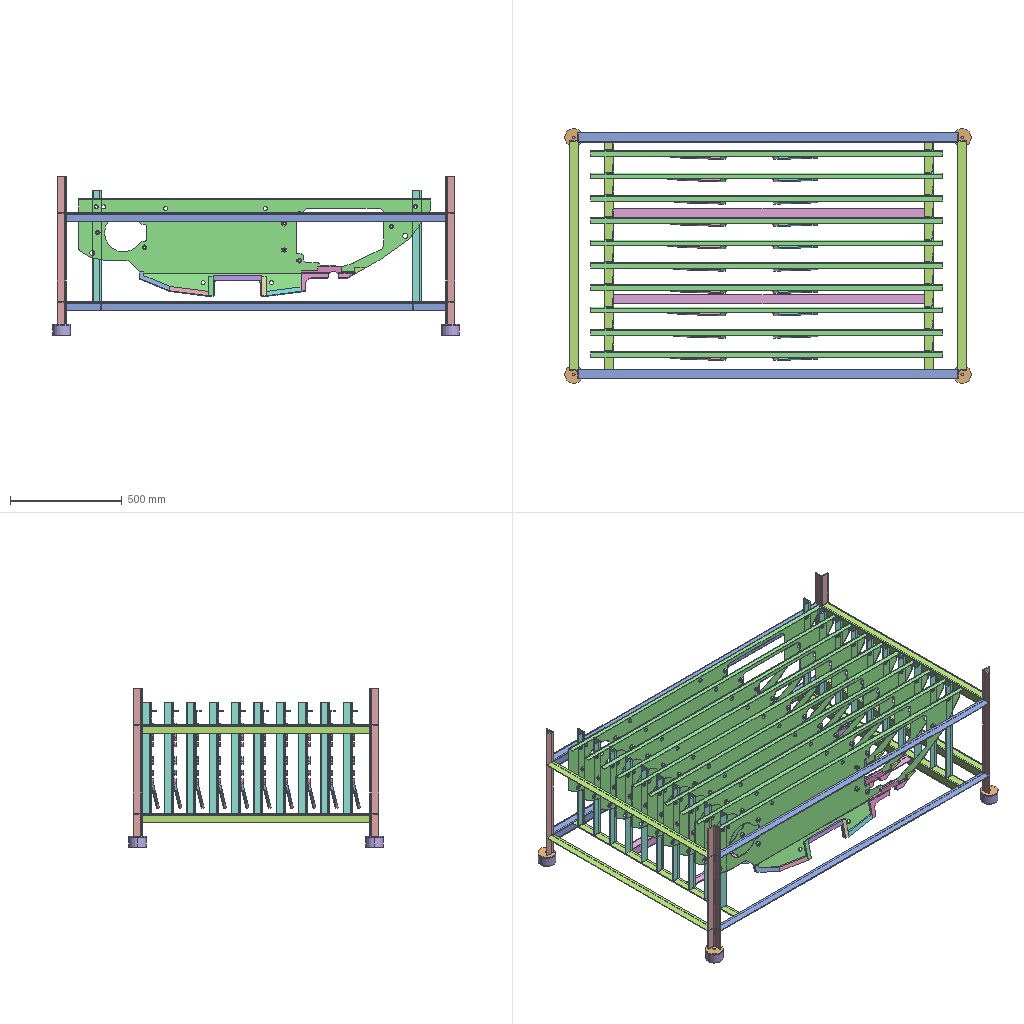Assembly | SolidWorks | 9 different items | 55 placed | box 1820 x 1139 x 710 mm
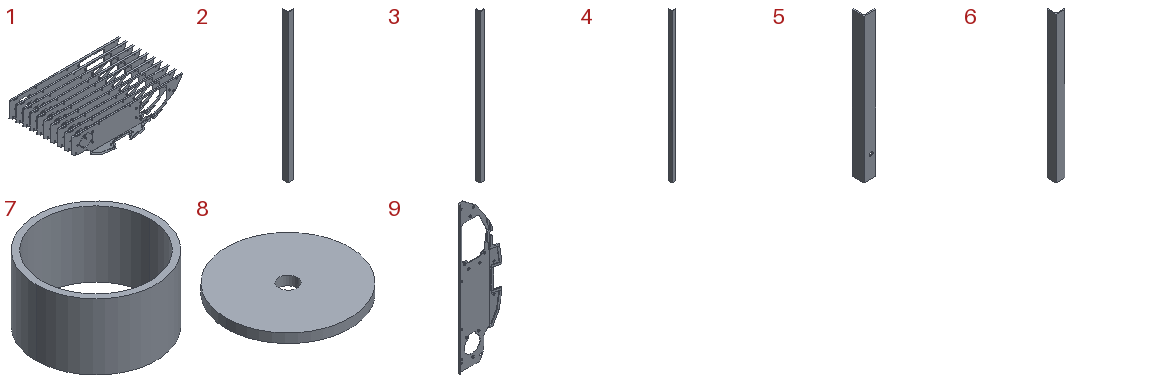Parts list (item | name | quantity | parent item | size | volume | features):
1 | (subassembly) | x1 | - | - | - | features ReferencePattern 9, LocalLPattern 1
2 | - | x6 | - | 40 x 40 x 1020 mm | 314774 mm3 | features Extrusion 1
3 | - | x2 | - | 40 x 40 x 1389 mm | 428648 mm3 | features Extrusion 1
4 | - | x4 | - | 40 x 40 x 1700 mm | 524623 mm3 | features Extrusion 1
5 | - | x20 | - | 40 x 40 x 500 mm | 153770 mm3 | features Extrusion 1, ICE 1
6 | - | x4 | - | 40 x 40 x 660 mm | 203677 mm3 | features Extrusion 1
7 | - | x4 | - | 80 x 80 x 44 mm | 42022 mm3 | features Extrusion 1
8 | - | x4 | - | 80 x 80 x 6 mm | 29481 mm3 | features FlatPattern 1, SMBaseFlange 1, SheetMetal 1
9 | - | x10 | in 1 | - | - | features BaseBody 17, RefSurface 8
Mates (type | each side: item.copy, entity, surface, feature):
Coincident | 6.1 face plane Boss-Extrude1 | 4.1 face plane Boss-Extrude1 | 2 times
DistanceDim | 6.1 face plane Boss-Extrude1 | 4.1 face plane Boss-Extrude1
Coincident | 6.1 face plane Boss-Extrude1 | 2.1 face plane Boss-Extrude1 | 2 times
Coincident | 4.1 face plane Boss-Extrude1 | 2.1 face plane Boss-Extrude1
Coincident | 2.1 face plane Boss-Extrude1 | 6.2 face plane Boss-Extrude1 | 2 times
Coincident | 6.1 face plane Boss-Extrude1 | 6.2 face plane Boss-Extrude1
Coincident | 6.2 face plane Boss-Extrude1 | 4.2 face plane Boss-Extrude1 | 2 times
Coincident | 2.1 face plane Boss-Extrude1 | 4.2 face plane Boss-Extrude1
Coincident | 4.2 face plane Boss-Extrude1 | 6.3 face plane Boss-Extrude1 | 2 times
Coincident | 6.2 face plane Boss-Extrude1 | 6.3 face plane Boss-Extrude1
Coincident | 6.3 face plane Boss-Extrude1 | 2.2 face plane Boss-Extrude1 | 2 times
Coincident | 4.2 face plane Boss-Extrude1 | 2.2 face plane Boss-Extrude1
Coincident | 2.2 face plane Boss-Extrude1 | 6.4 face plane Boss-Extrude1
Coincident | 4.1 face plane Boss-Extrude1 | 6.4 face plane Boss-Extrude1
Coincident | 6.3 face plane Boss-Extrude1 | 6.4 face plane Boss-Extrude1
Coincident | 4.1 face plane Boss-Extrude1 | 2.3 face plane Boss-Extrude1 | 2 times
DistanceDim | 2.1 face plane Boss-Extrude1 | 2.3 face plane Boss-Extrude1
Coincident | 2.2 face plane Boss-Extrude1 | 2.4 face plane Boss-Extrude1
DistanceDim | 2.2 face plane Boss-Extrude1 | 2.4 face plane Boss-Extrude1
Coincident | 4.1 face plane Boss-Extrude1 | 2.4 face plane Boss-Extrude1
Coincident | 2.4 face plane Boss-Extrude1 | 3.1 face plane Boss-Extrude1
Coincident | 2.3 face plane Boss-Extrude1 | 3.1 face plane Boss-Extrude1
DistanceDim | 4.1 face plane Boss-Extrude1 | 3.1 face plane Boss-Extrude1
Coincident | 2.4 face plane Boss-Extrude1 | 3.2 face plane Boss-Extrude1 | 2 times
DistanceDim | 4.2 face plane Boss-Extrude1 | 3.2 face plane Boss-Extrude1
Coincident | 2.3 face plane Boss-Extrude1 | 5.1 face plane Boss-Extrude1 | 2 times
Coincident | 4.1 face plane Boss-Extrude1 | 5.1 face plane Boss-Extrude1
Coincident | 5.1 face plane Boss-Extrude1 | 9.1 face plane 22P-54-36131_ASM.stp-1/22P-54-36131-01.stp-1-solid1
Concentric | 5.1 face cylinder Cut-Extrude1 | 9.1 face cylinder 22P-54-36131_ASM.stp-1/22P-54-36131-01.stp-1-solid1
Coincident | 6.1 face plane Boss-Extrude1 | 8.1 face plane Base-Flange1
DistanceDim | 8.1 face cylinder Base-Flange1 | 6.1 face plane Boss-Extrude1
DistanceDim | 6.1 face plane Boss-Extrude1 | 8.1 face cylinder Base-Flange1
Concentric | 8.1 face cylinder Base-Flange1 | 7.1 face cylinder Boss-Extrude1
Coincident | 8.1 face plane Base-Flange1 | 7.1 face plane Boss-Extrude1